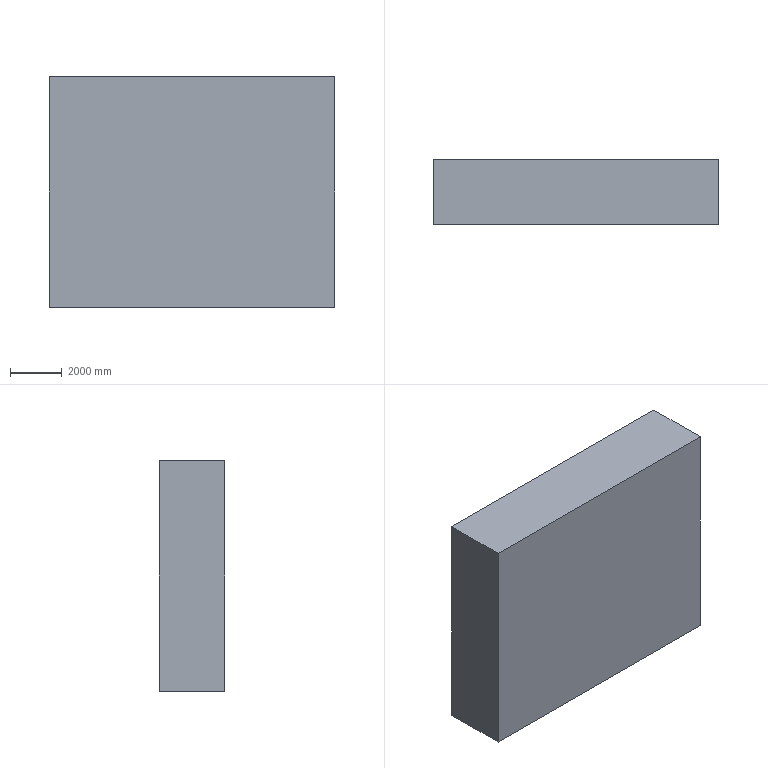Part | STEP file | Concrete | 1 solid | 39 faces | box 11000 x 2521 x 8890 mm | volume 220029236509 mm3 | plane 39